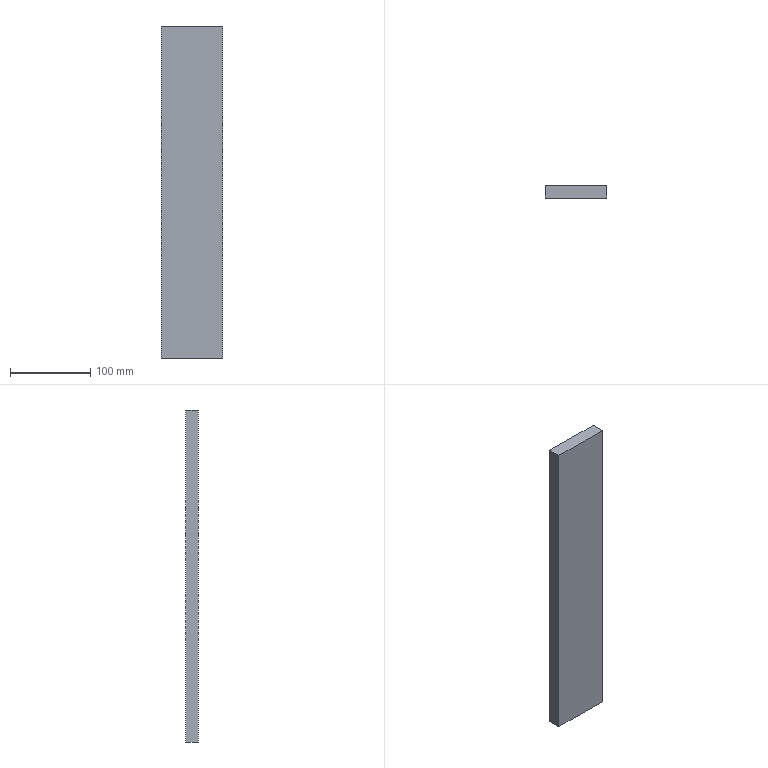Part | SolidWorks | features BaseBody 1 | 1 solid | 6 faces | box 76 x 16 x 413.5 mm | volume 502816 mm3 | plane 6
STEP:
#1=CARTESIAN_POINT('',(53.889,24.883,0.));
#2=VERTEX_POINT('',#1);
#3=CARTESIAN_POINT('',(-22.111,24.883,0.));
#4=VERTEX_POINT('',#3);
#5=CARTESIAN_POINT('',(-22.111,24.883,0.));
#6=DIRECTION('',(-1.,0.,0.));
#7=VECTOR('',#6,1000.);
#8=LINE('',#5,#7);
#9=EDGE_CURVE('',#2,#4,#8,.T.);
#10=ORIENTED_EDGE('',*,*,#9,.T.);
#11=CARTESIAN_POINT('',(-22.111,24.883,413.5));
#12=VERTEX_POINT('',#11);
#13=CARTESIAN_POINT('',(-22.111,24.883,0.));
#14=DIRECTION('',(0.,0.,1.));
#15=VECTOR('',#14,1000.);
#16=LINE('',#13,#15);
#17=EDGE_CURVE('',#4,#12,#16,.T.);
#18=ORIENTED_EDGE('',*,*,#17,.T.);
#19=CARTESIAN_POINT('',(53.889,24.883,413.5));
#20=VERTEX_POINT('',#19);
#21=CARTESIAN_POINT('',(-22.111,24.883,413.5));
#22=DIRECTION('',(1.,0.,0.));
#23=VECTOR('',#22,1000.);
#24=LINE('',#21,#23);
#25=EDGE_CURVE('',#12,#20,#24,.T.);
#26=ORIENTED_EDGE('',*,*,#25,.T.);
#27=CARTESIAN_POINT('',(53.889,24.883,0.));
#28=DIRECTION('',(0.,0.,-1.));
#29=VECTOR('',#28,1000.);
#30=LINE('',#27,#29);
#31=EDGE_CURVE('',#20,#2,#30,.T.);
#32=ORIENTED_EDGE('',*,*,#31,.T.);
#33=EDGE_LOOP('',(#10,#18,#26,#32));
#34=FACE_OUTER_BOUND('',#33,.T.);
#35=CARTESIAN_POINT('',(-22.111,24.883,0.));
#36=DIRECTION('',(0.,1.,0.));
#37=DIRECTION('',(-1.,0.,0.));
#38=AXIS2_PLACEMENT_3D('',#35,#36,#37);
#39=PLANE('',#38);
#40=ADVANCED_FACE('',(#34),#39,.T.);
#41=CARTESIAN_POINT('',(-22.111,8.883,0.));
#42=VERTEX_POINT('',#41);
#43=CARTESIAN_POINT('',(-22.111,8.883,0.));
#44=DIRECTION('',(0.,-1.,0.));
#45=VECTOR('',#44,1000.);
#46=LINE('',#43,#45);
#47=EDGE_CURVE('',#4,#42,#46,.T.);
#48=ORIENTED_EDGE('',*,*,#47,.T.);
#49=CARTESIAN_POINT('',(-22.111,8.883,413.5));
#50=VERTEX_POINT('',#49);
#51=CARTESIAN_POINT('',(-22.111,8.883,0.));
#52=DIRECTION('',(0.,0.,1.));
#53=VECTOR('',#52,1000.);
#54=LINE('',#51,#53);
#55=EDGE_CURVE('',#42,#50,#54,.T.);
#56=ORIENTED_EDGE('',*,*,#55,.T.);
#57=CARTESIAN_POINT('',(-22.111,8.883,413.5));
#58=DIRECTION('',(0.,1.,0.));
#59=VECTOR('',#58,1000.);
#60=LINE('',#57,#59);
#61=EDGE_CURVE('',#50,#12,#60,.T.);
#62=ORIENTED_EDGE('',*,*,#61,.T.);
#63=ORIENTED_EDGE('',*,*,#17,.F.);
#64=EDGE_LOOP('',(#48,#56,#62,#63));
#65=FACE_OUTER_BOUND('',#64,.T.);
#66=CARTESIAN_POINT('',(-22.111,8.883,0.));
#67=DIRECTION('',(-1.,0.,0.));
#68=DIRECTION('',(0.,-1.,0.));
#69=AXIS2_PLACEMENT_3D('',#66,#67,#68);
#70=PLANE('',#69);
#71=ADVANCED_FACE('',(#65),#70,.T.);
#72=CARTESIAN_POINT('',(53.889,8.883,0.));
#73=VERTEX_POINT('',#72);
#74=CARTESIAN_POINT('',(53.889,16.883,0.));
#75=DIRECTION('',(0.,1.,0.));
#76=VECTOR('',#75,1000.);
#77=LINE('',#74,#76);
#78=EDGE_CURVE('',#73,#2,#77,.T.);
#79=ORIENTED_EDGE('',*,*,#78,.F.);
#80=CARTESIAN_POINT('',(15.889,8.883,0.));
#81=DIRECTION('',(1.,0.,0.));
#82=VECTOR('',#81,1000.);
#83=LINE('',#80,#82);
#84=EDGE_CURVE('',#42,#73,#83,.T.);
#85=ORIENTED_EDGE('',*,*,#84,.F.);
#86=ORIENTED_EDGE('',*,*,#47,.F.);
#87=ORIENTED_EDGE('',*,*,#9,.F.);
#88=EDGE_LOOP('',(#79,#85,#86,#87));
#89=FACE_OUTER_BOUND('',#88,.T.);
#90=CARTESIAN_POINT('',(15.889,16.883,0.));
#91=DIRECTION('',(0.,0.,1.));
#92=DIRECTION('',(1.,0.,0.));
#93=AXIS2_PLACEMENT_3D('',#90,#91,#92);
#94=PLANE('',#93);
#95=ADVANCED_FACE('',(#89),#94,.F.);
#96=ORIENTED_EDGE('',*,*,#78,.T.);
#97=ORIENTED_EDGE('',*,*,#31,.F.);
#98=CARTESIAN_POINT('',(53.889,8.883,413.5));
#99=VERTEX_POINT('',#98);
#100=CARTESIAN_POINT('',(53.889,24.883,413.5));
#101=DIRECTION('',(0.,-1.,0.));
#102=VECTOR('',#101,1000.);
#103=LINE('',#100,#102);
#104=EDGE_CURVE('',#20,#99,#103,.T.);
#105=ORIENTED_EDGE('',*,*,#104,.T.);
#106=CARTESIAN_POINT('',(53.889,8.883,0.));
#107=DIRECTION('',(0.,0.,-1.));
#108=VECTOR('',#107,1000.);
#109=LINE('',#106,#108);
#110=EDGE_CURVE('',#99,#73,#109,.T.);
#111=ORIENTED_EDGE('',*,*,#110,.T.);
#112=EDGE_LOOP('',(#96,#97,#105,#111));
#113=FACE_OUTER_BOUND('',#112,.T.);
#114=CARTESIAN_POINT('',(53.889,24.883,0.));
#115=DIRECTION('',(1.,0.,0.));
#116=DIRECTION('',(0.,0.,-1.));
#117=AXIS2_PLACEMENT_3D('',#114,#115,#116);
#118=PLANE('',#117);
#119=ADVANCED_FACE('',(#113),#118,.T.);
#120=ORIENTED_EDGE('',*,*,#61,.F.);
#121=CARTESIAN_POINT('',(15.889,8.883,413.5));
#122=DIRECTION('',(1.,0.,0.));
#123=VECTOR('',#122,1000.);
#124=LINE('',#121,#123);
#125=EDGE_CURVE('',#50,#99,#124,.T.);
#126=ORIENTED_EDGE('',*,*,#125,.T.);
#127=ORIENTED_EDGE('',*,*,#104,.F.);
#128=ORIENTED_EDGE('',*,*,#25,.F.);
#129=EDGE_LOOP('',(#120,#126,#127,#128));
#130=FACE_OUTER_BOUND('',#129,.T.);
#131=CARTESIAN_POINT('',(15.889,16.883,413.5));
#132=DIRECTION('',(0.,0.,1.));
#133=DIRECTION('',(1.,0.,0.));
#134=AXIS2_PLACEMENT_3D('',#131,#132,#133);
#135=PLANE('',#134);
#136=ADVANCED_FACE('',(#130),#135,.T.);
#137=ORIENTED_EDGE('',*,*,#84,.T.);
#138=ORIENTED_EDGE('',*,*,#110,.F.);
#139=ORIENTED_EDGE('',*,*,#125,.F.);
#140=ORIENTED_EDGE('',*,*,#55,.F.);
#141=EDGE_LOOP('',(#137,#138,#139,#140));
#142=FACE_OUTER_BOUND('',#141,.T.);
#143=CARTESIAN_POINT('',(53.889,8.883,0.));
#144=DIRECTION('',(0.,-1.,0.));
#145=DIRECTION('',(1.,0.,0.));
#146=AXIS2_PLACEMENT_3D('',#143,#144,#145);
#147=PLANE('',#146);
#148=ADVANCED_FACE('',(#142),#147,.T.);
#149=CLOSED_SHELL('',(#40,#71,#95,#119,#136,#148));
#150=MANIFOLD_SOLID_BREP('',#149);
#151=CARTESIAN_POINT('',(0.,0.,0.));
#152=DIRECTION('',(0.,0.,1.));
#153=DIRECTION('',(1.,0.,0.));
#154=AXIS2_PLACEMENT_3D('',#151,#152,#153);
#155=(LENGTH_UNIT()NAMED_UNIT(*)SI_UNIT(.MILLI.,.METRE.));
#156=UNCERTAINTY_MEASURE_WITH_UNIT(LENGTH_MEASURE(0.00001),#155,'','');
#157=(NAMED_UNIT(*)PLANE_ANGLE_UNIT()SI_UNIT($,.RADIAN.));
#158=(NAMED_UNIT(*)SI_UNIT($,.STERADIAN.)SOLID_ANGLE_UNIT());
#159=(GEOMETRIC_REPRESENTATION_CONTEXT(3)GLOBAL_UNCERTAINTY_ASSIGNED_CONTEXT((#156))GLOBAL_UNIT_ASSIGNED_CONTEXT((#155,#157,#158))REPRESENTATION_CONTEXT('',''));
#160=ADVANCED_BREP_SHAPE_REPRESENTATION('',(#150,#154),#159);